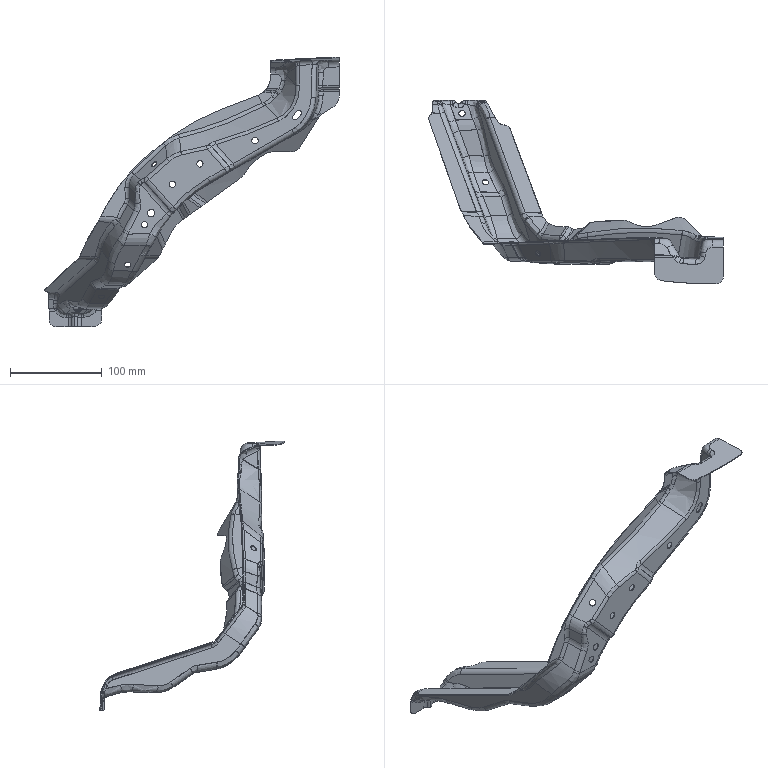Part | 1 solid | 512 faces | box 321.591 x 201.087 x 294.399 mm | volume 46877 mm3 | spline 291 | cylinder 140 | plane 64 | sphere 12 | other 5 | commonest cylinder face diameters 10 x29 11.6 x20 7 x16 16 x11 20 x10 8.4 x9